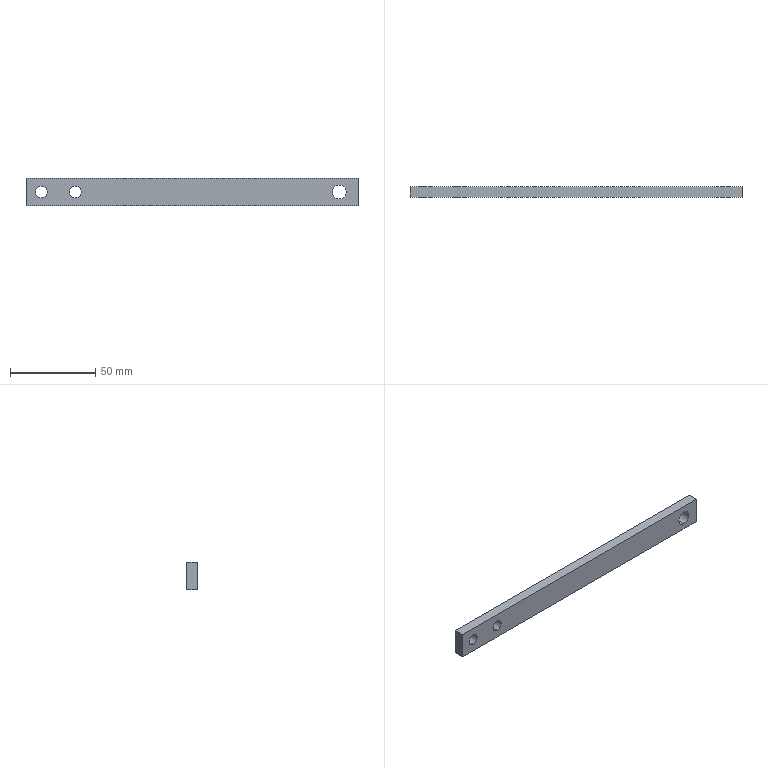Part | SolidWorks | features BaseBody 1 | 1 solid | 12 faces | box 195 x 6 x 16 mm | volume 17967 mm3 | cylinder 6 | plane 6 | commonest cylinder face diameters 6.8 x4 8.2 x2
STEP:
#1=CARTESIAN_POINT('',(86.5,0.,-4.1));
#2=VERTEX_POINT('',#1);
#3=CARTESIAN_POINT('',(86.5,0.,4.1));
#4=VERTEX_POINT('',#3);
#5=CARTESIAN_POINT('',(86.5,0.,0.));
#6=DIRECTION('',(0.,1.,0.));
#7=DIRECTION('',(0.,0.,1.));
#8=AXIS2_PLACEMENT_3D('',#5,#6,#7);
#9=CIRCLE('',#8,4.1);
#10=EDGE_CURVE('',#2,#4,#9,.T.);
#11=ORIENTED_EDGE('',*,*,#10,.F.);
#12=CARTESIAN_POINT('',(86.5,6.,-4.1));
#13=VERTEX_POINT('',#12);
#14=CARTESIAN_POINT('',(86.5,0.,-4.1));
#15=DIRECTION('',(0.,1.,0.));
#16=VECTOR('',#15,1000.);
#17=LINE('',#14,#16);
#18=EDGE_CURVE('',#2,#13,#17,.T.);
#19=ORIENTED_EDGE('',*,*,#18,.T.);
#20=CARTESIAN_POINT('',(86.5,6.,4.1));
#21=VERTEX_POINT('',#20);
#22=CARTESIAN_POINT('',(86.5,6.,0.));
#23=DIRECTION('',(0.,1.,0.));
#24=DIRECTION('',(0.,0.,1.));
#25=AXIS2_PLACEMENT_3D('',#22,#23,#24);
#26=CIRCLE('',#25,4.1);
#27=EDGE_CURVE('',#13,#21,#26,.T.);
#28=ORIENTED_EDGE('',*,*,#27,.T.);
#29=CARTESIAN_POINT('',(86.5,0.,4.1));
#30=DIRECTION('',(0.,1.,0.));
#31=VECTOR('',#30,1000.);
#32=LINE('',#29,#31);
#33=EDGE_CURVE('',#4,#21,#32,.T.);
#34=ORIENTED_EDGE('',*,*,#33,.F.);
#35=EDGE_LOOP('',(#11,#19,#28,#34));
#36=FACE_OUTER_BOUND('',#35,.T.);
#37=CARTESIAN_POINT('',(86.5,0.,0.));
#38=DIRECTION('',(0.,1.,0.));
#39=DIRECTION('',(0.,0.,1.));
#40=AXIS2_PLACEMENT_3D('',#37,#38,#39);
#41=CYLINDRICAL_SURFACE('',#40,4.1);
#42=ADVANCED_FACE('',(#36),#41,.F.);
#43=CARTESIAN_POINT('',(-68.5,0.,-3.4));
#44=VERTEX_POINT('',#43);
#45=CARTESIAN_POINT('',(-68.5,0.,3.4));
#46=VERTEX_POINT('',#45);
#47=CARTESIAN_POINT('',(-68.5,0.,0.));
#48=DIRECTION('',(0.,1.,0.));
#49=DIRECTION('',(0.,0.,1.));
#50=AXIS2_PLACEMENT_3D('',#47,#48,#49);
#51=CIRCLE('',#50,3.4);
#52=EDGE_CURVE('',#44,#46,#51,.T.);
#53=ORIENTED_EDGE('',*,*,#52,.F.);
#54=CARTESIAN_POINT('',(-68.5,6.,-3.4));
#55=VERTEX_POINT('',#54);
#56=CARTESIAN_POINT('',(-68.5,0.,-3.4));
#57=DIRECTION('',(0.,1.,0.));
#58=VECTOR('',#57,1000.);
#59=LINE('',#56,#58);
#60=EDGE_CURVE('',#44,#55,#59,.T.);
#61=ORIENTED_EDGE('',*,*,#60,.T.);
#62=CARTESIAN_POINT('',(-68.5,6.,3.4));
#63=VERTEX_POINT('',#62);
#64=CARTESIAN_POINT('',(-68.5,6.,0.));
#65=DIRECTION('',(0.,1.,0.));
#66=DIRECTION('',(0.,0.,1.));
#67=AXIS2_PLACEMENT_3D('',#64,#65,#66);
#68=CIRCLE('',#67,3.4);
#69=EDGE_CURVE('',#55,#63,#68,.T.);
#70=ORIENTED_EDGE('',*,*,#69,.T.);
#71=CARTESIAN_POINT('',(-68.5,0.,3.4));
#72=DIRECTION('',(0.,1.,0.));
#73=VECTOR('',#72,1000.);
#74=LINE('',#71,#73);
#75=EDGE_CURVE('',#46,#63,#74,.T.);
#76=ORIENTED_EDGE('',*,*,#75,.F.);
#77=EDGE_LOOP('',(#53,#61,#70,#76));
#78=FACE_OUTER_BOUND('',#77,.T.);
#79=CARTESIAN_POINT('',(-68.5,0.,0.));
#80=DIRECTION('',(0.,1.,0.));
#81=DIRECTION('',(0.,0.,1.));
#82=AXIS2_PLACEMENT_3D('',#79,#80,#81);
#83=CYLINDRICAL_SURFACE('',#82,3.4);
#84=ADVANCED_FACE('',(#78),#83,.F.);
#85=CARTESIAN_POINT('',(-88.5,0.,-3.4));
#86=VERTEX_POINT('',#85);
#87=CARTESIAN_POINT('',(-88.5,0.,3.4));
#88=VERTEX_POINT('',#87);
#89=CARTESIAN_POINT('',(-88.5,0.,0.));
#90=DIRECTION('',(0.,1.,0.));
#91=DIRECTION('',(0.,0.,1.));
#92=AXIS2_PLACEMENT_3D('',#89,#90,#91);
#93=CIRCLE('',#92,3.4);
#94=EDGE_CURVE('',#86,#88,#93,.T.);
#95=ORIENTED_EDGE('',*,*,#94,.F.);
#96=CARTESIAN_POINT('',(-88.5,6.,-3.4));
#97=VERTEX_POINT('',#96);
#98=CARTESIAN_POINT('',(-88.5,0.,-3.4));
#99=DIRECTION('',(0.,1.,0.));
#100=VECTOR('',#99,1000.);
#101=LINE('',#98,#100);
#102=EDGE_CURVE('',#86,#97,#101,.T.);
#103=ORIENTED_EDGE('',*,*,#102,.T.);
#104=CARTESIAN_POINT('',(-88.5,6.,3.4));
#105=VERTEX_POINT('',#104);
#106=CARTESIAN_POINT('',(-88.5,6.,0.));
#107=DIRECTION('',(0.,1.,0.));
#108=DIRECTION('',(0.,0.,1.));
#109=AXIS2_PLACEMENT_3D('',#106,#107,#108);
#110=CIRCLE('',#109,3.4);
#111=EDGE_CURVE('',#97,#105,#110,.T.);
#112=ORIENTED_EDGE('',*,*,#111,.T.);
#113=CARTESIAN_POINT('',(-88.5,0.,3.4));
#114=DIRECTION('',(0.,1.,0.));
#115=VECTOR('',#114,1000.);
#116=LINE('',#113,#115);
#117=EDGE_CURVE('',#88,#105,#116,.T.);
#118=ORIENTED_EDGE('',*,*,#117,.F.);
#119=EDGE_LOOP('',(#95,#103,#112,#118));
#120=FACE_OUTER_BOUND('',#119,.T.);
#121=CARTESIAN_POINT('',(-88.5,0.,0.));
#122=DIRECTION('',(0.,1.,0.));
#123=DIRECTION('',(0.,0.,1.));
#124=AXIS2_PLACEMENT_3D('',#121,#122,#123);
#125=CYLINDRICAL_SURFACE('',#124,3.4);
#126=ADVANCED_FACE('',(#120),#125,.F.);
#127=CARTESIAN_POINT('',(-97.5,6.,-8.));
#128=VERTEX_POINT('',#127);
#129=CARTESIAN_POINT('',(97.5,6.,-8.));
#130=VERTEX_POINT('',#129);
#131=CARTESIAN_POINT('',(0.,6.,-8.));
#132=DIRECTION('',(1.,0.,0.));
#133=VECTOR('',#132,1000.);
#134=LINE('',#131,#133);
#135=EDGE_CURVE('',#128,#130,#134,.T.);
#136=ORIENTED_EDGE('',*,*,#135,.F.);
#137=CARTESIAN_POINT('',(-97.5,6.,8.));
#138=VERTEX_POINT('',#137);
#139=CARTESIAN_POINT('',(-97.5,6.,0.));
#140=DIRECTION('',(0.,0.,-1.));
#141=VECTOR('',#140,1000.);
#142=LINE('',#139,#141);
#143=EDGE_CURVE('',#138,#128,#142,.T.);
#144=ORIENTED_EDGE('',*,*,#143,.F.);
#145=CARTESIAN_POINT('',(97.5,6.,8.));
#146=VERTEX_POINT('',#145);
#147=CARTESIAN_POINT('',(0.,6.,8.));
#148=DIRECTION('',(-1.,0.,0.));
#149=VECTOR('',#148,1000.);
#150=LINE('',#147,#149);
#151=EDGE_CURVE('',#146,#138,#150,.T.);
#152=ORIENTED_EDGE('',*,*,#151,.F.);
#153=CARTESIAN_POINT('',(97.5,6.,0.));
#154=DIRECTION('',(0.,0.,1.));
#155=VECTOR('',#154,1000.);
#156=LINE('',#153,#155);
#157=EDGE_CURVE('',#130,#146,#156,.T.);
#158=ORIENTED_EDGE('',*,*,#157,.F.);
#159=EDGE_LOOP('',(#136,#144,#152,#158));
#160=FACE_OUTER_BOUND('',#159,.T.);
#161=CARTESIAN_POINT('',(86.5,6.,0.));
#162=DIRECTION('',(0.,1.,0.));
#163=DIRECTION('',(0.,0.,1.));
#164=AXIS2_PLACEMENT_3D('',#161,#162,#163);
#165=CIRCLE('',#164,4.1);
#166=EDGE_CURVE('',#21,#13,#165,.T.);
#167=ORIENTED_EDGE('',*,*,#166,.F.);
#168=ORIENTED_EDGE('',*,*,#27,.F.);
#169=EDGE_LOOP('',(#167,#168));
#170=FACE_BOUND('',#169,.T.);
#171=CARTESIAN_POINT('',(-68.5,6.,0.));
#172=DIRECTION('',(0.,1.,0.));
#173=DIRECTION('',(0.,0.,1.));
#174=AXIS2_PLACEMENT_3D('',#171,#172,#173);
#175=CIRCLE('',#174,3.4);
#176=EDGE_CURVE('',#63,#55,#175,.T.);
#177=ORIENTED_EDGE('',*,*,#176,.F.);
#178=ORIENTED_EDGE('',*,*,#69,.F.);
#179=EDGE_LOOP('',(#177,#178));
#180=FACE_BOUND('',#179,.T.);
#181=CARTESIAN_POINT('',(-88.5,6.,0.));
#182=DIRECTION('',(0.,1.,0.));
#183=DIRECTION('',(0.,0.,1.));
#184=AXIS2_PLACEMENT_3D('',#181,#182,#183);
#185=CIRCLE('',#184,3.4);
#186=EDGE_CURVE('',#105,#97,#185,.T.);
#187=ORIENTED_EDGE('',*,*,#186,.F.);
#188=ORIENTED_EDGE('',*,*,#111,.F.);
#189=EDGE_LOOP('',(#187,#188));
#190=FACE_BOUND('',#189,.T.);
#191=CARTESIAN_POINT('',(0.,6.,0.));
#192=DIRECTION('',(0.,-1.,0.));
#193=DIRECTION('',(0.,0.,-1.));
#194=AXIS2_PLACEMENT_3D('',#191,#192,#193);
#195=PLANE('',#194);
#196=ADVANCED_FACE('',(#160,#170,#180,#190),#195,.F.);
#197=CARTESIAN_POINT('',(97.5,0.,-8.));
#198=VERTEX_POINT('',#197);
#199=CARTESIAN_POINT('',(97.5,6.,-8.));
#200=DIRECTION('',(0.,-1.,0.));
#201=VECTOR('',#200,1000.);
#202=LINE('',#199,#201);
#203=EDGE_CURVE('',#130,#198,#202,.T.);
#204=ORIENTED_EDGE('',*,*,#203,.F.);
#205=ORIENTED_EDGE('',*,*,#157,.T.);
#206=CARTESIAN_POINT('',(97.5,0.,8.));
#207=VERTEX_POINT('',#206);
#208=CARTESIAN_POINT('',(97.5,6.,8.));
#209=DIRECTION('',(0.,1.,0.));
#210=VECTOR('',#209,1000.);
#211=LINE('',#208,#210);
#212=EDGE_CURVE('',#207,#146,#211,.T.);
#213=ORIENTED_EDGE('',*,*,#212,.F.);
#214=CARTESIAN_POINT('',(97.5,0.,8.));
#215=DIRECTION('',(0.,0.,1.));
#216=VECTOR('',#215,1000.);
#217=LINE('',#214,#216);
#218=EDGE_CURVE('',#198,#207,#217,.T.);
#219=ORIENTED_EDGE('',*,*,#218,.F.);
#220=EDGE_LOOP('',(#204,#205,#213,#219));
#221=FACE_OUTER_BOUND('',#220,.T.);
#222=CARTESIAN_POINT('',(97.5,6.,8.));
#223=DIRECTION('',(-1.,0.,0.));
#224=DIRECTION('',(0.,0.,1.));
#225=AXIS2_PLACEMENT_3D('',#222,#223,#224);
#226=PLANE('',#225);
#227=ADVANCED_FACE('',(#221),#226,.F.);
#228=CARTESIAN_POINT('',(-97.5,0.,-8.));
#229=VERTEX_POINT('',#228);
#230=CARTESIAN_POINT('',(-97.5,6.,-8.));
#231=DIRECTION('',(0.,-1.,0.));
#232=VECTOR('',#231,1000.);
#233=LINE('',#230,#232);
#234=EDGE_CURVE('',#128,#229,#233,.T.);
#235=ORIENTED_EDGE('',*,*,#234,.F.);
#236=ORIENTED_EDGE('',*,*,#135,.T.);
#237=ORIENTED_EDGE('',*,*,#203,.T.);
#238=CARTESIAN_POINT('',(-97.5,0.,-8.));
#239=DIRECTION('',(1.,0.,0.));
#240=VECTOR('',#239,1000.);
#241=LINE('',#238,#240);
#242=EDGE_CURVE('',#229,#198,#241,.T.);
#243=ORIENTED_EDGE('',*,*,#242,.F.);
#244=EDGE_LOOP('',(#235,#236,#237,#243));
#245=FACE_OUTER_BOUND('',#244,.T.);
#246=CARTESIAN_POINT('',(-97.5,6.,-8.));
#247=DIRECTION('',(0.,0.,1.));
#248=DIRECTION('',(1.,0.,0.));
#249=AXIS2_PLACEMENT_3D('',#246,#247,#248);
#250=PLANE('',#249);
#251=ADVANCED_FACE('',(#245),#250,.F.);
#252=CARTESIAN_POINT('',(-97.5,0.,8.));
#253=VERTEX_POINT('',#252);
#254=CARTESIAN_POINT('',(-97.5,6.,8.));
#255=DIRECTION('',(0.,-1.,0.));
#256=VECTOR('',#255,1000.);
#257=LINE('',#254,#256);
#258=EDGE_CURVE('',#138,#253,#257,.T.);
#259=ORIENTED_EDGE('',*,*,#258,.F.);
#260=ORIENTED_EDGE('',*,*,#143,.T.);
#261=ORIENTED_EDGE('',*,*,#234,.T.);
#262=CARTESIAN_POINT('',(-97.5,0.,8.));
#263=DIRECTION('',(0.,0.,-1.));
#264=VECTOR('',#263,1000.);
#265=LINE('',#262,#264);
#266=EDGE_CURVE('',#253,#229,#265,.T.);
#267=ORIENTED_EDGE('',*,*,#266,.F.);
#268=EDGE_LOOP('',(#259,#260,#261,#267));
#269=FACE_OUTER_BOUND('',#268,.T.);
#270=CARTESIAN_POINT('',(-97.5,6.,8.));
#271=DIRECTION('',(1.,0.,0.));
#272=DIRECTION('',(0.,0.,-1.));
#273=AXIS2_PLACEMENT_3D('',#270,#271,#272);
#274=PLANE('',#273);
#275=ADVANCED_FACE('',(#269),#274,.F.);
#276=ORIENTED_EDGE('',*,*,#212,.T.);
#277=ORIENTED_EDGE('',*,*,#151,.T.);
#278=ORIENTED_EDGE('',*,*,#258,.T.);
#279=CARTESIAN_POINT('',(-97.5,0.,8.));
#280=DIRECTION('',(-1.,0.,0.));
#281=VECTOR('',#280,1000.);
#282=LINE('',#279,#281);
#283=EDGE_CURVE('',#207,#253,#282,.T.);
#284=ORIENTED_EDGE('',*,*,#283,.F.);
#285=EDGE_LOOP('',(#276,#277,#278,#284));
#286=FACE_OUTER_BOUND('',#285,.T.);
#287=CARTESIAN_POINT('',(-97.5,6.,8.));
#288=DIRECTION('',(0.,0.,-1.));
#289=DIRECTION('',(-1.,0.,0.));
#290=AXIS2_PLACEMENT_3D('',#287,#288,#289);
#291=PLANE('',#290);
#292=ADVANCED_FACE('',(#286),#291,.F.);
#293=ORIENTED_EDGE('',*,*,#18,.F.);
#294=CARTESIAN_POINT('',(86.5,0.,0.));
#295=DIRECTION('',(0.,1.,0.));
#296=DIRECTION('',(0.,0.,1.));
#297=AXIS2_PLACEMENT_3D('',#294,#295,#296);
#298=CIRCLE('',#297,4.1);
#299=EDGE_CURVE('',#4,#2,#298,.T.);
#300=ORIENTED_EDGE('',*,*,#299,.F.);
#301=ORIENTED_EDGE('',*,*,#33,.T.);
#302=ORIENTED_EDGE('',*,*,#166,.T.);
#303=EDGE_LOOP('',(#293,#300,#301,#302));
#304=FACE_OUTER_BOUND('',#303,.T.);
#305=CARTESIAN_POINT('',(86.5,0.,0.));
#306=DIRECTION('',(0.,1.,0.));
#307=DIRECTION('',(0.,0.,1.));
#308=AXIS2_PLACEMENT_3D('',#305,#306,#307);
#309=CYLINDRICAL_SURFACE('',#308,4.1);
#310=ADVANCED_FACE('',(#304),#309,.F.);
#311=ORIENTED_EDGE('',*,*,#60,.F.);
#312=CARTESIAN_POINT('',(-68.5,0.,0.));
#313=DIRECTION('',(0.,1.,0.));
#314=DIRECTION('',(0.,0.,1.));
#315=AXIS2_PLACEMENT_3D('',#312,#313,#314);
#316=CIRCLE('',#315,3.4);
#317=EDGE_CURVE('',#46,#44,#316,.T.);
#318=ORIENTED_EDGE('',*,*,#317,.F.);
#319=ORIENTED_EDGE('',*,*,#75,.T.);
#320=ORIENTED_EDGE('',*,*,#176,.T.);
#321=EDGE_LOOP('',(#311,#318,#319,#320));
#322=FACE_OUTER_BOUND('',#321,.T.);
#323=CARTESIAN_POINT('',(-68.5,0.,0.));
#324=DIRECTION('',(0.,1.,0.));
#325=DIRECTION('',(0.,0.,1.));
#326=AXIS2_PLACEMENT_3D('',#323,#324,#325);
#327=CYLINDRICAL_SURFACE('',#326,3.4);
#328=ADVANCED_FACE('',(#322),#327,.F.);
#329=ORIENTED_EDGE('',*,*,#102,.F.);
#330=CARTESIAN_POINT('',(-88.5,0.,0.));
#331=DIRECTION('',(0.,1.,0.));
#332=DIRECTION('',(0.,0.,1.));
#333=AXIS2_PLACEMENT_3D('',#330,#331,#332);
#334=CIRCLE('',#333,3.4);
#335=EDGE_CURVE('',#88,#86,#334,.T.);
#336=ORIENTED_EDGE('',*,*,#335,.F.);
#337=ORIENTED_EDGE('',*,*,#117,.T.);
#338=ORIENTED_EDGE('',*,*,#186,.T.);
#339=EDGE_LOOP('',(#329,#336,#337,#338));
#340=FACE_OUTER_BOUND('',#339,.T.);
#341=CARTESIAN_POINT('',(-88.5,0.,0.));
#342=DIRECTION('',(0.,1.,0.));
#343=DIRECTION('',(0.,0.,1.));
#344=AXIS2_PLACEMENT_3D('',#341,#342,#343);
#345=CYLINDRICAL_SURFACE('',#344,3.4);
#346=ADVANCED_FACE('',(#340),#345,.F.);
#347=ORIENTED_EDGE('',*,*,#266,.T.);
#348=ORIENTED_EDGE('',*,*,#242,.T.);
#349=ORIENTED_EDGE('',*,*,#218,.T.);
#350=ORIENTED_EDGE('',*,*,#283,.T.);
#351=EDGE_LOOP('',(#347,#348,#349,#350));
#352=FACE_OUTER_BOUND('',#351,.T.);
#353=ORIENTED_EDGE('',*,*,#299,.T.);
#354=ORIENTED_EDGE('',*,*,#10,.T.);
#355=EDGE_LOOP('',(#353,#354));
#356=FACE_BOUND('',#355,.T.);
#357=ORIENTED_EDGE('',*,*,#317,.T.);
#358=ORIENTED_EDGE('',*,*,#52,.T.);
#359=EDGE_LOOP('',(#357,#358));
#360=FACE_BOUND('',#359,.T.);
#361=ORIENTED_EDGE('',*,*,#335,.T.);
#362=ORIENTED_EDGE('',*,*,#94,.T.);
#363=EDGE_LOOP('',(#361,#362));
#364=FACE_BOUND('',#363,.T.);
#365=CARTESIAN_POINT('',(0.,0.,0.));
#366=DIRECTION('',(0.,-1.,0.));
#367=DIRECTION('',(0.,0.,-1.));
#368=AXIS2_PLACEMENT_3D('',#365,#366,#367);
#369=PLANE('',#368);
#370=ADVANCED_FACE('',(#352,#356,#360,#364),#369,.T.);
#371=CLOSED_SHELL('',(#42,#84,#126,#196,#227,#251,#275,#292,#310,#328,#346,#370));
#372=MANIFOLD_SOLID_BREP('',#371);
#373=CARTESIAN_POINT('',(0.,0.,0.));
#374=DIRECTION('',(0.,0.,1.));
#375=DIRECTION('',(1.,0.,0.));
#376=AXIS2_PLACEMENT_3D('',#373,#374,#375);
#377=(LENGTH_UNIT()NAMED_UNIT(*)SI_UNIT(.MILLI.,.METRE.));
#378=UNCERTAINTY_MEASURE_WITH_UNIT(LENGTH_MEASURE(0.00001),#377,'','');
#379=(NAMED_UNIT(*)PLANE_ANGLE_UNIT()SI_UNIT($,.RADIAN.));
#380=(NAMED_UNIT(*)SI_UNIT($,.STERADIAN.)SOLID_ANGLE_UNIT());
#381=(GEOMETRIC_REPRESENTATION_CONTEXT(3)GLOBAL_UNCERTAINTY_ASSIGNED_CONTEXT((#378))GLOBAL_UNIT_ASSIGNED_CONTEXT((#377,#379,#380))REPRESENTATION_CONTEXT('',''));
#382=ADVANCED_BREP_SHAPE_REPRESENTATION('',(#372,#376),#381);